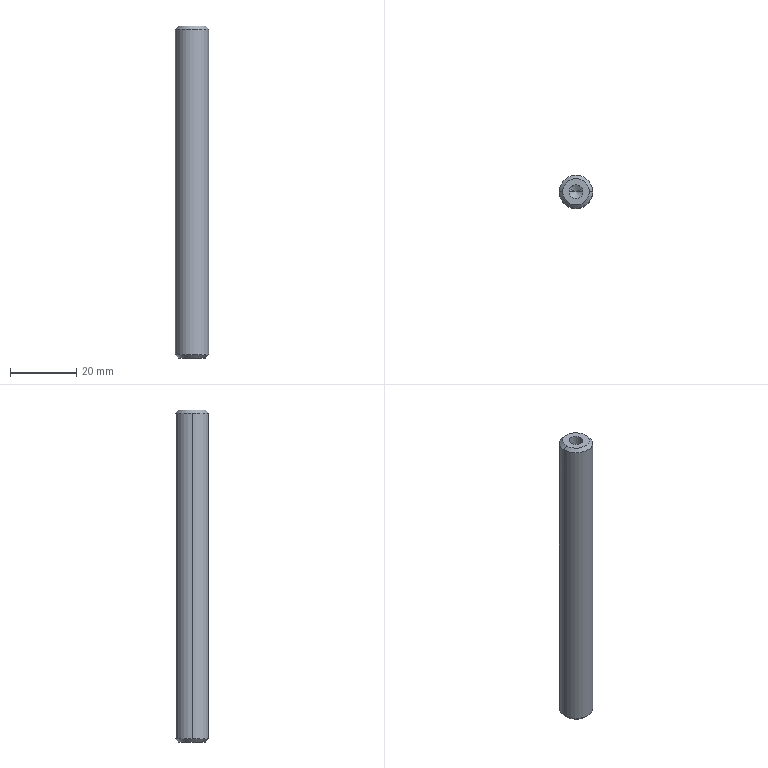Part | SolidWorks | features Revolution 1 | 1 solid | 16 faces | box 10 x 10 x 100 mm | volume 7469 mm3 | cone 8 | cylinder 6 | plane 2 | commonest cylinder face diameters 4.2 x4 10 x2